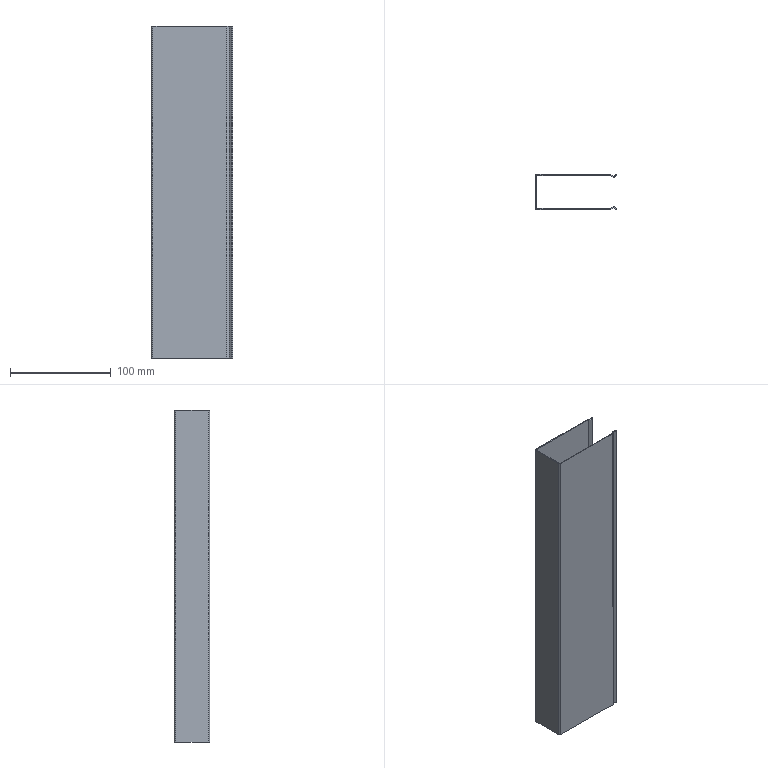Part | STEP file | Cable trough 35_L330 | 1 solid | 22 faces | box 80.625 x 35 x 330 mm | volume 64629 mm3 | plane 18 | cylinder 4 | commonest cylinder face diameters 1 x2 3 x2